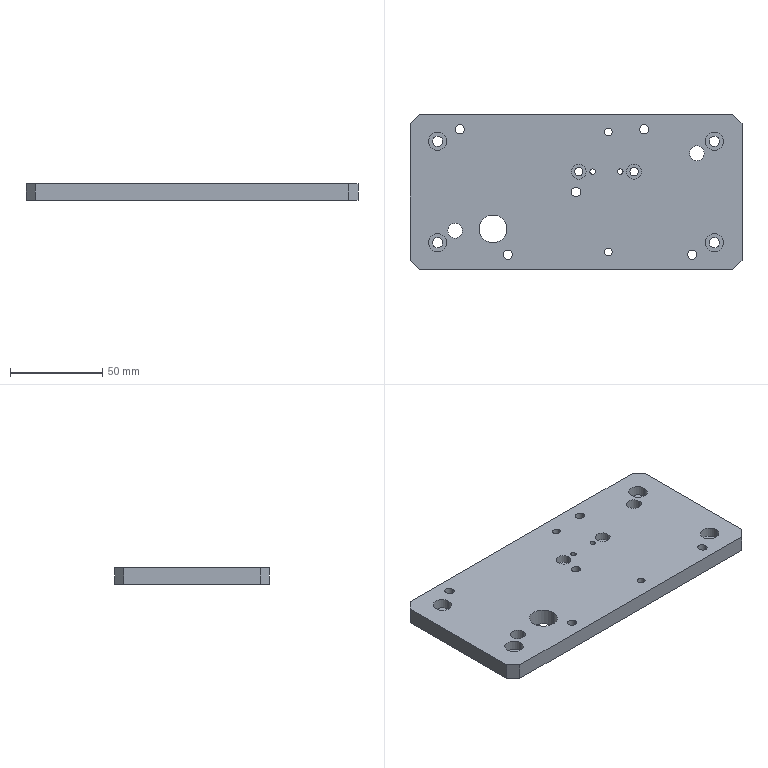Part | STEP file | PN_0034 | 1 solid | 64 faces | box 180 x 84 x 9 mm | volume 129247 mm3 | cylinder 48 | plane 16 | commonest cylinder face diameters 5 x10 5.5 x8 8 x8 10 x8 3 x4 4.2 x4